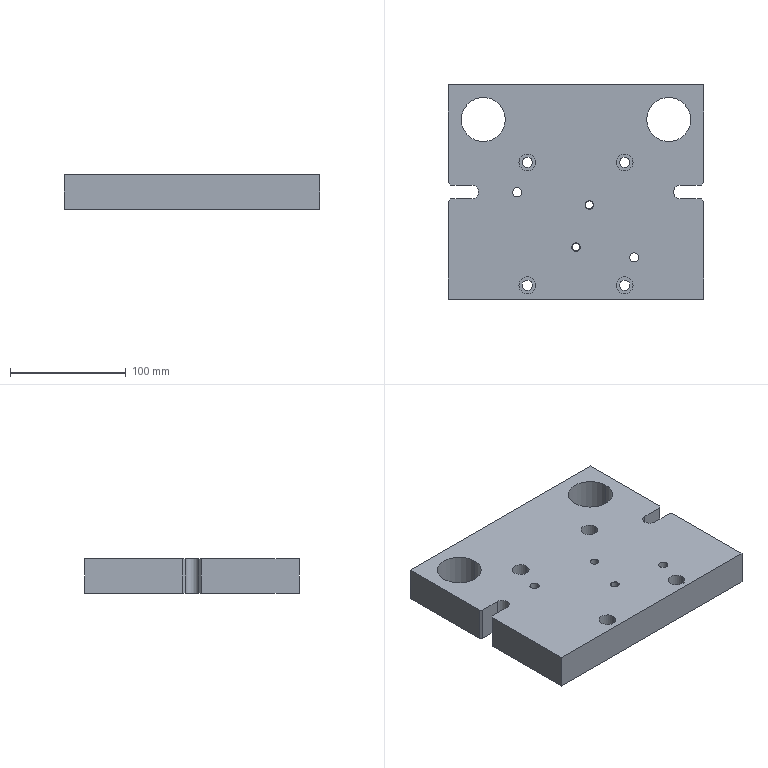Part | SolidWorks | features BaseBody 1, MoveFace 1 | 1 solid | 55 faces | box 220 x 185 x 30 mm | volume 1117612 mm3 | cylinder 31 | plane 20 | cone 4 | commonest cylinder face diameters 9.007 x8 14.5 x8 6.805 x4 8 x4 38 x4 12 x3